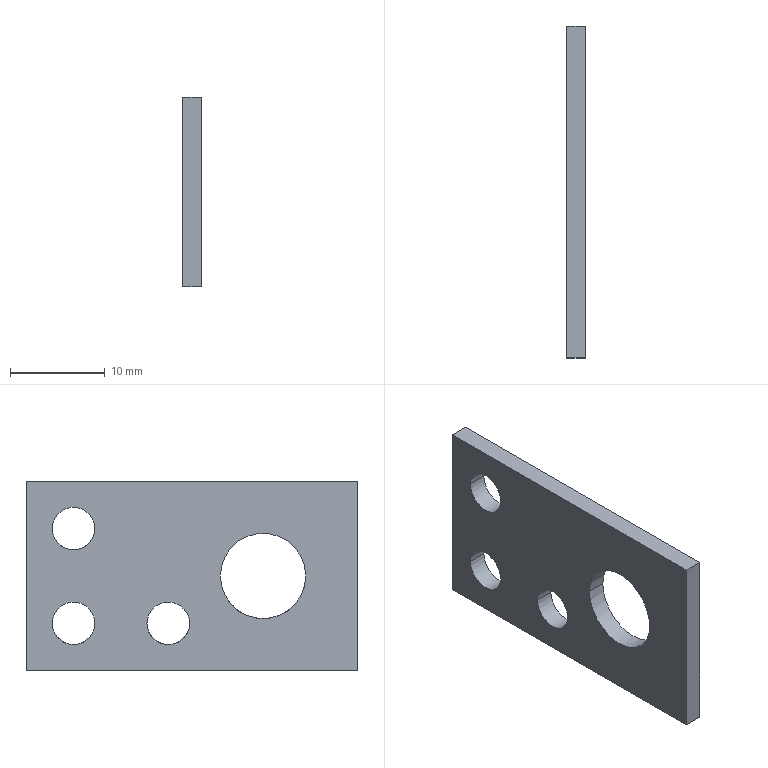Part | Creo | 1 solid | 14 faces | box 2 x 35 x 20 mm | volume 1177 mm3 | cylinder 8 | plane 6 | commonest cylinder face diameters 4.5 x6 9 x2
STEP:
#1=CARTESIAN_POINT('',(-302.,-15.429,-177.999));
#2=VERTEX_POINT('',#1);
#3=CARTESIAN_POINT('',(-302.,-50.429,-177.999));
#4=VERTEX_POINT('',#3);
#5=CARTESIAN_POINT('',(-302.,-15.429,-177.999));
#6=DIRECTION('',(0.,-1.,0.));
#7=VECTOR('',#6,35.);
#8=LINE('',#5,#7);
#9=EDGE_CURVE('',#2,#4,#8,.T.);
#10=ORIENTED_EDGE('',*,*,#9,.T.);
#11=CARTESIAN_POINT('',(-302.,-50.429,-197.999));
#12=VERTEX_POINT('',#11);
#13=CARTESIAN_POINT('',(-302.,-50.429,-197.999));
#14=DIRECTION('',(0.,0.,1.));
#15=VECTOR('',#14,20.);
#16=LINE('',#13,#15);
#17=EDGE_CURVE('',#12,#4,#16,.T.);
#18=ORIENTED_EDGE('',*,*,#17,.F.);
#19=CARTESIAN_POINT('',(-302.,-15.429,-197.999));
#20=VERTEX_POINT('',#19);
#21=CARTESIAN_POINT('',(-302.,-50.429,-197.999));
#22=DIRECTION('',(0.,1.,0.));
#23=VECTOR('',#22,35.);
#24=LINE('',#21,#23);
#25=EDGE_CURVE('',#12,#20,#24,.T.);
#26=ORIENTED_EDGE('',*,*,#25,.T.);
#27=CARTESIAN_POINT('',(-302.,-15.429,-197.999));
#28=DIRECTION('',(0.,0.,1.));
#29=VECTOR('',#28,20.);
#30=LINE('',#27,#29);
#31=EDGE_CURVE('',#20,#2,#30,.T.);
#32=ORIENTED_EDGE('',*,*,#31,.T.);
#33=EDGE_LOOP('',(#10,#18,#26,#32));
#34=FACE_OUTER_BOUND('',#33,.F.);
#35=CARTESIAN_POINT('',(-302.,-44.929,-187.999));
#36=VERTEX_POINT('',#35);
#37=CARTESIAN_POINT('',(-302.,-35.929,-187.999));
#38=VERTEX_POINT('',#37);
#39=CARTESIAN_POINT('',(-302.,-40.429,-187.999));
#40=DIRECTION('',(1.,0.,0.));
#41=DIRECTION('',(0.,-1.,0.));
#42=AXIS2_PLACEMENT_3D('',#39,#40,#41);
#43=CIRCLE('',#42,4.5);
#44=EDGE_CURVE('',#36,#38,#43,.T.);
#45=ORIENTED_EDGE('',*,*,#44,.F.);
#46=CARTESIAN_POINT('',(-302.,-40.429,-187.999));
#47=DIRECTION('',(1.,0.,0.));
#48=DIRECTION('',(0.,1.,0.));
#49=AXIS2_PLACEMENT_3D('',#46,#47,#48);
#50=CIRCLE('',#49,4.5);
#51=EDGE_CURVE('',#38,#36,#50,.T.);
#52=ORIENTED_EDGE('',*,*,#51,.F.);
#53=EDGE_LOOP('',(#45,#52));
#54=FACE_BOUND('',#53,.F.);
#55=CARTESIAN_POINT('',(-302.,-22.679,-192.999));
#56=VERTEX_POINT('',#55);
#57=CARTESIAN_POINT('',(-302.,-18.179,-192.999));
#58=VERTEX_POINT('',#57);
#59=CARTESIAN_POINT('',(-302.,-20.429,-192.999));
#60=DIRECTION('',(1.,0.,0.));
#61=DIRECTION('',(0.,-1.,0.));
#62=AXIS2_PLACEMENT_3D('',#59,#60,#61);
#63=CIRCLE('',#62,2.25);
#64=EDGE_CURVE('',#56,#58,#63,.T.);
#65=ORIENTED_EDGE('',*,*,#64,.F.);
#66=CARTESIAN_POINT('',(-302.,-20.429,-192.999));
#67=DIRECTION('',(1.,0.,0.));
#68=DIRECTION('',(0.,1.,0.));
#69=AXIS2_PLACEMENT_3D('',#66,#67,#68);
#70=CIRCLE('',#69,2.25);
#71=EDGE_CURVE('',#58,#56,#70,.T.);
#72=ORIENTED_EDGE('',*,*,#71,.F.);
#73=EDGE_LOOP('',(#65,#72));
#74=FACE_BOUND('',#73,.F.);
#75=CARTESIAN_POINT('',(-302.,-32.679,-192.999));
#76=VERTEX_POINT('',#75);
#77=CARTESIAN_POINT('',(-302.,-28.179,-192.999));
#78=VERTEX_POINT('',#77);
#79=CARTESIAN_POINT('',(-302.,-30.429,-192.999));
#80=DIRECTION('',(1.,0.,0.));
#81=DIRECTION('',(0.,-1.,0.));
#82=AXIS2_PLACEMENT_3D('',#79,#80,#81);
#83=CIRCLE('',#82,2.25);
#84=EDGE_CURVE('',#76,#78,#83,.T.);
#85=ORIENTED_EDGE('',*,*,#84,.F.);
#86=CARTESIAN_POINT('',(-302.,-30.429,-192.999));
#87=DIRECTION('',(1.,0.,0.));
#88=DIRECTION('',(0.,1.,0.));
#89=AXIS2_PLACEMENT_3D('',#86,#87,#88);
#90=CIRCLE('',#89,2.25);
#91=EDGE_CURVE('',#78,#76,#90,.T.);
#92=ORIENTED_EDGE('',*,*,#91,.F.);
#93=EDGE_LOOP('',(#85,#92));
#94=FACE_BOUND('',#93,.F.);
#95=CARTESIAN_POINT('',(-302.,-22.679,-182.999));
#96=VERTEX_POINT('',#95);
#97=CARTESIAN_POINT('',(-302.,-18.179,-182.999));
#98=VERTEX_POINT('',#97);
#99=CARTESIAN_POINT('',(-302.,-20.429,-182.999));
#100=DIRECTION('',(1.,0.,0.));
#101=DIRECTION('',(0.,-1.,0.));
#102=AXIS2_PLACEMENT_3D('',#99,#100,#101);
#103=CIRCLE('',#102,2.25);
#104=EDGE_CURVE('',#96,#98,#103,.T.);
#105=ORIENTED_EDGE('',*,*,#104,.F.);
#106=CARTESIAN_POINT('',(-302.,-20.429,-182.999));
#107=DIRECTION('',(1.,0.,0.));
#108=DIRECTION('',(0.,1.,0.));
#109=AXIS2_PLACEMENT_3D('',#106,#107,#108);
#110=CIRCLE('',#109,2.25);
#111=EDGE_CURVE('',#98,#96,#110,.T.);
#112=ORIENTED_EDGE('',*,*,#111,.F.);
#113=EDGE_LOOP('',(#105,#112));
#114=FACE_BOUND('',#113,.F.);
#115=CARTESIAN_POINT('',(-302.,-32.929,-177.999));
#116=DIRECTION('',(-1.,0.,0.));
#117=DIRECTION('',(0.,0.,1.));
#118=AXIS2_PLACEMENT_3D('',#115,#116,#117);
#119=PLANE('',#118);
#120=ADVANCED_FACE('',(#34,#54,#74,#94,#114),#119,.T.);
#121=CARTESIAN_POINT('',(-300.,-18.179,-192.999));
#122=VERTEX_POINT('',#121);
#123=CARTESIAN_POINT('',(-300.,-20.429,-195.249));
#124=VERTEX_POINT('',#123);
#125=CARTESIAN_POINT('',(-300.,-20.429,-192.999));
#126=DIRECTION('',(-1.,0.,0.));
#127=DIRECTION('',(0.,1.,0.));
#128=AXIS2_PLACEMENT_3D('',#125,#126,#127);
#129=CIRCLE('',#128,2.25);
#130=EDGE_CURVE('',#122,#124,#129,.T.);
#131=ORIENTED_EDGE('',*,*,#130,.T.);
#132=CARTESIAN_POINT('',(-300.,-22.679,-192.999));
#133=VERTEX_POINT('',#132);
#134=CARTESIAN_POINT('',(-300.,-20.429,-192.999));
#135=DIRECTION('',(-1.,0.,0.));
#136=DIRECTION('',(0.,0.,-1.));
#137=AXIS2_PLACEMENT_3D('',#134,#135,#136);
#138=CIRCLE('',#137,2.25);
#139=EDGE_CURVE('',#124,#133,#138,.T.);
#140=ORIENTED_EDGE('',*,*,#139,.T.);
#141=CARTESIAN_POINT('',(-302.,-22.679,-192.999));
#142=DIRECTION('',(1.,0.,0.));
#143=VECTOR('',#142,2.);
#144=LINE('',#141,#143);
#145=EDGE_CURVE('',#56,#133,#144,.T.);
#146=ORIENTED_EDGE('',*,*,#145,.F.);
#147=ORIENTED_EDGE('',*,*,#64,.T.);
#148=CARTESIAN_POINT('',(-302.,-18.179,-192.999));
#149=DIRECTION('',(1.,0.,0.));
#150=VECTOR('',#149,2.);
#151=LINE('',#148,#150);
#152=EDGE_CURVE('',#58,#122,#151,.T.);
#153=ORIENTED_EDGE('',*,*,#152,.T.);
#154=EDGE_LOOP('',(#131,#140,#146,#147,#153));
#155=FACE_OUTER_BOUND('',#154,.F.);
#156=CARTESIAN_POINT('',(-302.,-20.429,-192.999));
#157=DIRECTION('',(1.,0.,0.));
#158=DIRECTION('',(0.,-1.,0.));
#159=AXIS2_PLACEMENT_3D('',#156,#157,#158);
#160=CYLINDRICAL_SURFACE('',#159,2.25);
#161=ADVANCED_FACE('',(#155),#160,.F.);
#162=CARTESIAN_POINT('',(-300.,-50.429,-197.999));
#163=VERTEX_POINT('',#162);
#164=CARTESIAN_POINT('',(-300.,-50.429,-177.999));
#165=VERTEX_POINT('',#164);
#166=CARTESIAN_POINT('',(-300.,-50.429,-197.999));
#167=DIRECTION('',(0.,0.,1.));
#168=VECTOR('',#167,20.);
#169=LINE('',#166,#168);
#170=EDGE_CURVE('',#163,#165,#169,.T.);
#171=ORIENTED_EDGE('',*,*,#170,.T.);
#172=CARTESIAN_POINT('',(-300.,-15.429,-177.999));
#173=VERTEX_POINT('',#172);
#174=CARTESIAN_POINT('',(-300.,-50.429,-177.999));
#175=DIRECTION('',(0.,1.,0.));
#176=VECTOR('',#175,35.);
#177=LINE('',#174,#176);
#178=EDGE_CURVE('',#165,#173,#177,.T.);
#179=ORIENTED_EDGE('',*,*,#178,.T.);
#180=CARTESIAN_POINT('',(-300.,-15.429,-197.999));
#181=VERTEX_POINT('',#180);
#182=CARTESIAN_POINT('',(-300.,-15.429,-197.999));
#183=DIRECTION('',(0.,0.,1.));
#184=VECTOR('',#183,20.);
#185=LINE('',#182,#184);
#186=EDGE_CURVE('',#181,#173,#185,.T.);
#187=ORIENTED_EDGE('',*,*,#186,.F.);
#188=CARTESIAN_POINT('',(-300.,-15.429,-197.999));
#189=DIRECTION('',(0.,-1.,0.));
#190=VECTOR('',#189,35.);
#191=LINE('',#188,#190);
#192=EDGE_CURVE('',#181,#163,#191,.T.);
#193=ORIENTED_EDGE('',*,*,#192,.T.);
#194=EDGE_LOOP('',(#171,#179,#187,#193));
#195=FACE_OUTER_BOUND('',#194,.F.);
#196=ORIENTED_EDGE('',*,*,#139,.F.);
#197=ORIENTED_EDGE('',*,*,#130,.F.);
#198=CARTESIAN_POINT('',(-300.,-20.429,-192.999));
#199=DIRECTION('',(-1.,0.,0.));
#200=DIRECTION('',(0.,-1.,0.));
#201=AXIS2_PLACEMENT_3D('',#198,#199,#200);
#202=CIRCLE('',#201,2.25);
#203=EDGE_CURVE('',#133,#122,#202,.T.);
#204=ORIENTED_EDGE('',*,*,#203,.F.);
#205=EDGE_LOOP('',(#196,#197,#204));
#206=FACE_BOUND('',#205,.F.);
#207=CARTESIAN_POINT('',(-300.,-30.429,-195.249));
#208=VERTEX_POINT('',#207);
#209=CARTESIAN_POINT('',(-300.,-32.679,-192.999));
#210=VERTEX_POINT('',#209);
#211=CARTESIAN_POINT('',(-300.,-30.429,-192.999));
#212=DIRECTION('',(-1.,0.,0.));
#213=DIRECTION('',(0.,0.,-1.));
#214=AXIS2_PLACEMENT_3D('',#211,#212,#213);
#215=CIRCLE('',#214,2.25);
#216=EDGE_CURVE('',#208,#210,#215,.T.);
#217=ORIENTED_EDGE('',*,*,#216,.F.);
#218=CARTESIAN_POINT('',(-300.,-28.179,-192.999));
#219=VERTEX_POINT('',#218);
#220=CARTESIAN_POINT('',(-300.,-30.429,-192.999));
#221=DIRECTION('',(-1.,0.,0.));
#222=DIRECTION('',(0.,1.,0.));
#223=AXIS2_PLACEMENT_3D('',#220,#221,#222);
#224=CIRCLE('',#223,2.25);
#225=EDGE_CURVE('',#219,#208,#224,.T.);
#226=ORIENTED_EDGE('',*,*,#225,.F.);
#227=CARTESIAN_POINT('',(-300.,-30.429,-192.999));
#228=DIRECTION('',(-1.,0.,0.));
#229=DIRECTION('',(0.,-1.,0.));
#230=AXIS2_PLACEMENT_3D('',#227,#228,#229);
#231=CIRCLE('',#230,2.25);
#232=EDGE_CURVE('',#210,#219,#231,.T.);
#233=ORIENTED_EDGE('',*,*,#232,.F.);
#234=EDGE_LOOP('',(#217,#226,#233));
#235=FACE_BOUND('',#234,.F.);
#236=CARTESIAN_POINT('',(-300.,-40.429,-192.499));
#237=VERTEX_POINT('',#236);
#238=CARTESIAN_POINT('',(-300.,-44.929,-187.999));
#239=VERTEX_POINT('',#238);
#240=CARTESIAN_POINT('',(-300.,-40.429,-187.999));
#241=DIRECTION('',(-1.,0.,0.));
#242=DIRECTION('',(0.,0.,-1.));
#243=AXIS2_PLACEMENT_3D('',#240,#241,#242);
#244=CIRCLE('',#243,4.5);
#245=EDGE_CURVE('',#237,#239,#244,.T.);
#246=ORIENTED_EDGE('',*,*,#245,.F.);
#247=CARTESIAN_POINT('',(-300.,-35.929,-187.999));
#248=VERTEX_POINT('',#247);
#249=CARTESIAN_POINT('',(-300.,-40.429,-187.999));
#250=DIRECTION('',(-1.,0.,0.));
#251=DIRECTION('',(0.,1.,0.));
#252=AXIS2_PLACEMENT_3D('',#249,#250,#251);
#253=CIRCLE('',#252,4.5);
#254=EDGE_CURVE('',#248,#237,#253,.T.);
#255=ORIENTED_EDGE('',*,*,#254,.F.);
#256=CARTESIAN_POINT('',(-300.,-40.429,-187.999));
#257=DIRECTION('',(-1.,0.,0.));
#258=DIRECTION('',(0.,-1.,0.));
#259=AXIS2_PLACEMENT_3D('',#256,#257,#258);
#260=CIRCLE('',#259,4.5);
#261=EDGE_CURVE('',#239,#248,#260,.T.);
#262=ORIENTED_EDGE('',*,*,#261,.F.);
#263=EDGE_LOOP('',(#246,#255,#262));
#264=FACE_BOUND('',#263,.F.);
#265=CARTESIAN_POINT('',(-300.,-20.429,-185.249));
#266=VERTEX_POINT('',#265);
#267=CARTESIAN_POINT('',(-300.,-22.679,-182.999));
#268=VERTEX_POINT('',#267);
#269=CARTESIAN_POINT('',(-300.,-20.429,-182.999));
#270=DIRECTION('',(-1.,0.,0.));
#271=DIRECTION('',(0.,0.,-1.));
#272=AXIS2_PLACEMENT_3D('',#269,#270,#271);
#273=CIRCLE('',#272,2.25);
#274=EDGE_CURVE('',#266,#268,#273,.T.);
#275=ORIENTED_EDGE('',*,*,#274,.F.);
#276=CARTESIAN_POINT('',(-300.,-18.179,-182.999));
#277=VERTEX_POINT('',#276);
#278=CARTESIAN_POINT('',(-300.,-20.429,-182.999));
#279=DIRECTION('',(-1.,0.,0.));
#280=DIRECTION('',(0.,1.,0.));
#281=AXIS2_PLACEMENT_3D('',#278,#279,#280);
#282=CIRCLE('',#281,2.25);
#283=EDGE_CURVE('',#277,#266,#282,.T.);
#284=ORIENTED_EDGE('',*,*,#283,.F.);
#285=CARTESIAN_POINT('',(-300.,-20.429,-182.999));
#286=DIRECTION('',(-1.,0.,0.));
#287=DIRECTION('',(0.,-1.,0.));
#288=AXIS2_PLACEMENT_3D('',#285,#286,#287);
#289=CIRCLE('',#288,2.25);
#290=EDGE_CURVE('',#268,#277,#289,.T.);
#291=ORIENTED_EDGE('',*,*,#290,.F.);
#292=EDGE_LOOP('',(#275,#284,#291));
#293=FACE_BOUND('',#292,.F.);
#294=CARTESIAN_POINT('',(-300.,-32.929,-177.999));
#295=DIRECTION('',(1.,0.,0.));
#296=DIRECTION('',(0.,0.,-1.));
#297=AXIS2_PLACEMENT_3D('',#294,#295,#296);
#298=PLANE('',#297);
#299=ADVANCED_FACE('',(#195,#206,#235,#264,#293),#298,.T.);
#300=ORIENTED_EDGE('',*,*,#283,.T.);
#301=ORIENTED_EDGE('',*,*,#274,.T.);
#302=CARTESIAN_POINT('',(-302.,-22.679,-182.999));
#303=DIRECTION('',(1.,0.,0.));
#304=VECTOR('',#303,2.);
#305=LINE('',#302,#304);
#306=EDGE_CURVE('',#96,#268,#305,.T.);
#307=ORIENTED_EDGE('',*,*,#306,.F.);
#308=ORIENTED_EDGE('',*,*,#104,.T.);
#309=CARTESIAN_POINT('',(-302.,-18.179,-182.999));
#310=DIRECTION('',(1.,0.,0.));
#311=VECTOR('',#310,2.);
#312=LINE('',#309,#311);
#313=EDGE_CURVE('',#98,#277,#312,.T.);
#314=ORIENTED_EDGE('',*,*,#313,.T.);
#315=EDGE_LOOP('',(#300,#301,#307,#308,#314));
#316=FACE_OUTER_BOUND('',#315,.F.);
#317=CARTESIAN_POINT('',(-302.,-20.429,-182.999));
#318=DIRECTION('',(1.,0.,0.));
#319=DIRECTION('',(0.,-1.,0.));
#320=AXIS2_PLACEMENT_3D('',#317,#318,#319);
#321=CYLINDRICAL_SURFACE('',#320,2.25);
#322=ADVANCED_FACE('',(#316),#321,.F.);
#323=ORIENTED_EDGE('',*,*,#290,.T.);
#324=ORIENTED_EDGE('',*,*,#313,.F.);
#325=ORIENTED_EDGE('',*,*,#111,.T.);
#326=ORIENTED_EDGE('',*,*,#306,.T.);
#327=EDGE_LOOP('',(#323,#324,#325,#326));
#328=FACE_OUTER_BOUND('',#327,.F.);
#329=CARTESIAN_POINT('',(-302.,-20.429,-182.999));
#330=DIRECTION('',(1.,0.,0.));
#331=DIRECTION('',(0.,-1.,0.));
#332=AXIS2_PLACEMENT_3D('',#329,#330,#331);
#333=CYLINDRICAL_SURFACE('',#332,2.25);
#334=ADVANCED_FACE('',(#328),#333,.F.);
#335=ORIENTED_EDGE('',*,*,#203,.T.);
#336=ORIENTED_EDGE('',*,*,#152,.F.);
#337=ORIENTED_EDGE('',*,*,#71,.T.);
#338=ORIENTED_EDGE('',*,*,#145,.T.);
#339=EDGE_LOOP('',(#335,#336,#337,#338));
#340=FACE_OUTER_BOUND('',#339,.F.);
#341=CARTESIAN_POINT('',(-302.,-20.429,-192.999));
#342=DIRECTION('',(1.,0.,0.));
#343=DIRECTION('',(0.,-1.,0.));
#344=AXIS2_PLACEMENT_3D('',#341,#342,#343);
#345=CYLINDRICAL_SURFACE('',#344,2.25);
#346=ADVANCED_FACE('',(#340),#345,.F.);
#347=ORIENTED_EDGE('',*,*,#225,.T.);
#348=ORIENTED_EDGE('',*,*,#216,.T.);
#349=CARTESIAN_POINT('',(-302.,-32.679,-192.999));
#350=DIRECTION('',(1.,0.,0.));
#351=VECTOR('',#350,2.);
#352=LINE('',#349,#351);
#353=EDGE_CURVE('',#76,#210,#352,.T.);
#354=ORIENTED_EDGE('',*,*,#353,.F.);
#355=ORIENTED_EDGE('',*,*,#84,.T.);
#356=CARTESIAN_POINT('',(-302.,-28.179,-192.999));
#357=DIRECTION('',(1.,0.,0.));
#358=VECTOR('',#357,2.);
#359=LINE('',#356,#358);
#360=EDGE_CURVE('',#78,#219,#359,.T.);
#361=ORIENTED_EDGE('',*,*,#360,.T.);
#362=EDGE_LOOP('',(#347,#348,#354,#355,#361));
#363=FACE_OUTER_BOUND('',#362,.F.);
#364=CARTESIAN_POINT('',(-302.,-30.429,-192.999));
#365=DIRECTION('',(1.,0.,0.));
#366=DIRECTION('',(0.,-1.,0.));
#367=AXIS2_PLACEMENT_3D('',#364,#365,#366);
#368=CYLINDRICAL_SURFACE('',#367,2.25);
#369=ADVANCED_FACE('',(#363),#368,.F.);
#370=ORIENTED_EDGE('',*,*,#232,.T.);
#371=ORIENTED_EDGE('',*,*,#360,.F.);
#372=ORIENTED_EDGE('',*,*,#91,.T.);
#373=ORIENTED_EDGE('',*,*,#353,.T.);
#374=EDGE_LOOP('',(#370,#371,#372,#373));
#375=FACE_OUTER_BOUND('',#374,.F.);
#376=CARTESIAN_POINT('',(-302.,-30.429,-192.999));
#377=DIRECTION('',(1.,0.,0.));
#378=DIRECTION('',(0.,-1.,0.));
#379=AXIS2_PLACEMENT_3D('',#376,#377,#378);
#380=CYLINDRICAL_SURFACE('',#379,2.25);
#381=ADVANCED_FACE('',(#375),#380,.F.);
#382=ORIENTED_EDGE('',*,*,#254,.T.);
#383=ORIENTED_EDGE('',*,*,#245,.T.);
#384=CARTESIAN_POINT('',(-302.,-44.929,-187.999));
#385=DIRECTION('',(1.,0.,0.));
#386=VECTOR('',#385,2.);
#387=LINE('',#384,#386);
#388=EDGE_CURVE('',#36,#239,#387,.T.);
#389=ORIENTED_EDGE('',*,*,#388,.F.);
#390=ORIENTED_EDGE('',*,*,#44,.T.);
#391=CARTESIAN_POINT('',(-302.,-35.929,-187.999));
#392=DIRECTION('',(1.,0.,0.));
#393=VECTOR('',#392,2.);
#394=LINE('',#391,#393);
#395=EDGE_CURVE('',#38,#248,#394,.T.);
#396=ORIENTED_EDGE('',*,*,#395,.T.);
#397=EDGE_LOOP('',(#382,#383,#389,#390,#396));
#398=FACE_OUTER_BOUND('',#397,.F.);
#399=CARTESIAN_POINT('',(-302.,-40.429,-187.999));
#400=DIRECTION('',(1.,0.,0.));
#401=DIRECTION('',(0.,-1.,0.));
#402=AXIS2_PLACEMENT_3D('',#399,#400,#401);
#403=CYLINDRICAL_SURFACE('',#402,4.5);
#404=ADVANCED_FACE('',(#398),#403,.F.);
#405=ORIENTED_EDGE('',*,*,#261,.T.);
#406=ORIENTED_EDGE('',*,*,#395,.F.);
#407=ORIENTED_EDGE('',*,*,#51,.T.);
#408=ORIENTED_EDGE('',*,*,#388,.T.);
#409=EDGE_LOOP('',(#405,#406,#407,#408));
#410=FACE_OUTER_BOUND('',#409,.F.);
#411=CARTESIAN_POINT('',(-302.,-40.429,-187.999));
#412=DIRECTION('',(1.,0.,0.));
#413=DIRECTION('',(0.,-1.,0.));
#414=AXIS2_PLACEMENT_3D('',#411,#412,#413);
#415=CYLINDRICAL_SURFACE('',#414,4.5);
#416=ADVANCED_FACE('',(#410),#415,.F.);
#417=ORIENTED_EDGE('',*,*,#17,.T.);
#418=CARTESIAN_POINT('',(-302.,-50.429,-177.999));
#419=DIRECTION('',(1.,0.,0.));
#420=VECTOR('',#419,2.);
#421=LINE('',#418,#420);
#422=EDGE_CURVE('',#4,#165,#421,.T.);
#423=ORIENTED_EDGE('',*,*,#422,.T.);
#424=ORIENTED_EDGE('',*,*,#170,.F.);
#425=CARTESIAN_POINT('',(-300.,-50.429,-197.999));
#426=DIRECTION('',(-1.,0.,0.));
#427=VECTOR('',#426,2.);
#428=LINE('',#425,#427);
#429=EDGE_CURVE('',#163,#12,#428,.T.);
#430=ORIENTED_EDGE('',*,*,#429,.T.);
#431=EDGE_LOOP('',(#417,#423,#424,#430));
#432=FACE_OUTER_BOUND('',#431,.F.);
#433=CARTESIAN_POINT('',(-301.,-50.429,-177.999));
#434=DIRECTION('',(0.,-1.,0.));
#435=DIRECTION('',(0.,0.,1.));
#436=AXIS2_PLACEMENT_3D('',#433,#434,#435);
#437=PLANE('',#436);
#438=ADVANCED_FACE('',(#432),#437,.T.);
#439=ORIENTED_EDGE('',*,*,#9,.F.);
#440=CARTESIAN_POINT('',(-300.,-15.429,-177.999));
#441=DIRECTION('',(-1.,0.,0.));
#442=VECTOR('',#441,2.);
#443=LINE('',#440,#442);
#444=EDGE_CURVE('',#173,#2,#443,.T.);
#445=ORIENTED_EDGE('',*,*,#444,.F.);
#446=ORIENTED_EDGE('',*,*,#178,.F.);
#447=ORIENTED_EDGE('',*,*,#422,.F.);
#448=EDGE_LOOP('',(#439,#445,#446,#447));
#449=FACE_OUTER_BOUND('',#448,.F.);
#450=CARTESIAN_POINT('',(-301.,-32.929,-177.999));
#451=DIRECTION('',(0.,0.,1.));
#452=DIRECTION('',(1.,0.,0.));
#453=AXIS2_PLACEMENT_3D('',#450,#451,#452);
#454=PLANE('',#453);
#455=ADVANCED_FACE('',(#449),#454,.T.);
#456=ORIENTED_EDGE('',*,*,#186,.T.);
#457=ORIENTED_EDGE('',*,*,#444,.T.);
#458=ORIENTED_EDGE('',*,*,#31,.F.);
#459=CARTESIAN_POINT('',(-302.,-15.429,-197.999));
#460=DIRECTION('',(1.,0.,0.));
#461=VECTOR('',#460,2.);
#462=LINE('',#459,#461);
#463=EDGE_CURVE('',#20,#181,#462,.T.);
#464=ORIENTED_EDGE('',*,*,#463,.T.);
#465=EDGE_LOOP('',(#456,#457,#458,#464));
#466=FACE_OUTER_BOUND('',#465,.F.);
#467=CARTESIAN_POINT('',(-301.,-15.429,-177.999));
#468=DIRECTION('',(0.,1.,0.));
#469=DIRECTION('',(0.,0.,-1.));
#470=AXIS2_PLACEMENT_3D('',#467,#468,#469);
#471=PLANE('',#470);
#472=ADVANCED_FACE('',(#466),#471,.T.);
#473=ORIENTED_EDGE('',*,*,#429,.F.);
#474=ORIENTED_EDGE('',*,*,#192,.F.);
#475=ORIENTED_EDGE('',*,*,#463,.F.);
#476=ORIENTED_EDGE('',*,*,#25,.F.);
#477=EDGE_LOOP('',(#473,#474,#475,#476));
#478=FACE_OUTER_BOUND('',#477,.F.);
#479=CARTESIAN_POINT('',(-301.,-32.929,-197.999));
#480=DIRECTION('',(0.,0.,-1.));
#481=DIRECTION('',(-1.,0.,0.));
#482=AXIS2_PLACEMENT_3D('',#479,#480,#481);
#483=PLANE('',#482);
#484=ADVANCED_FACE('',(#478),#483,.T.);
#485=CLOSED_SHELL('',(#120,#161,#299,#322,#334,#346,#369,#381,#404,#416,#438,#455,#472,#484));
#486=MANIFOLD_SOLID_BREP('',#485);
#487=(LENGTH_UNIT()NAMED_UNIT(*)SI_UNIT(.MILLI.,.METRE.));
#488=UNCERTAINTY_MEASURE_WITH_UNIT(LENGTH_MEASURE(0.004036),#487,'','');
#489=(NAMED_UNIT(*)PLANE_ANGLE_UNIT()SI_UNIT($,.RADIAN.));
#490=PLANE_ANGLE_MEASURE_WITH_UNIT(PLANE_ANGLE_MEASURE(0.01745),#489);
#491=(CONVERSION_BASED_UNIT('DEGREE',#490)NAMED_UNIT(*)PLANE_ANGLE_UNIT());
#492=(NAMED_UNIT(*)SI_UNIT($,.STERADIAN.)SOLID_ANGLE_UNIT());
#493=(GEOMETRIC_REPRESENTATION_CONTEXT(3)GLOBAL_UNCERTAINTY_ASSIGNED_CONTEXT((#488))GLOBAL_UNIT_ASSIGNED_CONTEXT((#487,#491,#492))REPRESENTATION_CONTEXT('',''));
#494=ADVANCED_BREP_SHAPE_REPRESENTATION('',(#486),#493);